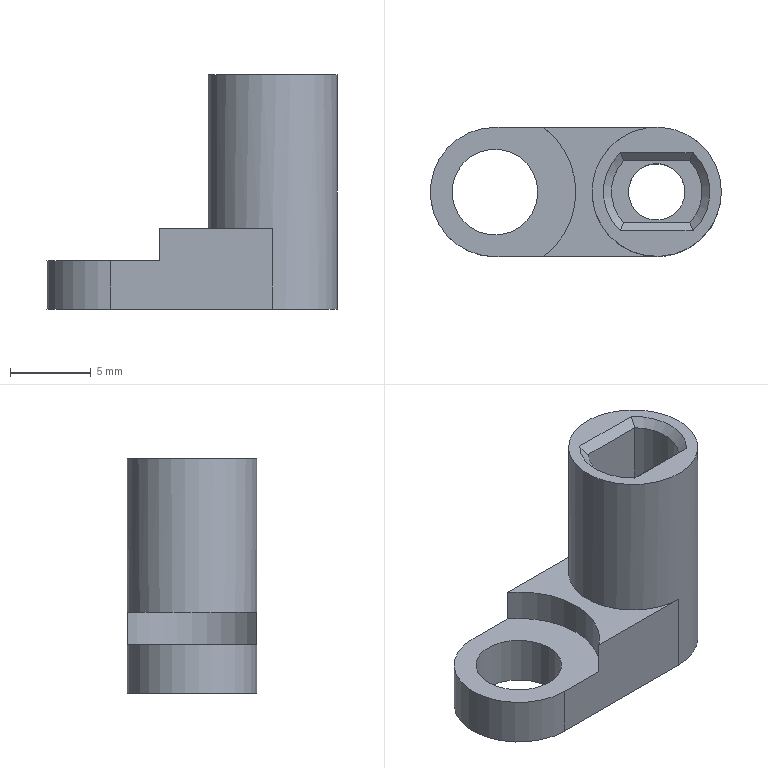Part | NX | features BREP 1 | 1 solid | 22 faces | box 18 x 8 x 14.5 mm | volume 713.021 mm3 | plane 12 | cylinder 8 | cone 2 | commonest cylinder face diameters 5.6 x2 8 x2 3.5 x1 5.3 x1 6 x1 10 x1
STEP:
#1=CARTESIAN_POINT('',(-20.737,0.,0.));
#2=VERTEX_POINT('',#1);
#3=CARTESIAN_POINT('',(-17.737,0.,0.));
#4=DIRECTION('',(0.,0.,-1.));
#5=DIRECTION('',(-1.,0.,0.));
#6=AXIS2_PLACEMENT_3D('',#3,#4,#5);
#7=CIRCLE('',#6,3.);
#8=EDGE_CURVE('',#2,#2,#7,.T.);
#9=ORIENTED_EDGE('',*,*,#8,.T.);
#10=EDGE_LOOP('',(#9));
#11=FACE_BOUND('',#10,.T.);
#12=CARTESIAN_POINT('',(-20.737,0.,2.));
#13=VERTEX_POINT('',#12);
#14=CARTESIAN_POINT('',(-17.737,0.,2.));
#15=DIRECTION('',(0.,0.,-1.));
#16=DIRECTION('',(-1.,0.,0.));
#17=AXIS2_PLACEMENT_3D('',#14,#15,#16);
#18=CIRCLE('',#17,3.);
#19=EDGE_CURVE('',#13,#13,#18,.T.);
#20=ORIENTED_EDGE('',*,*,#19,.F.);
#21=EDGE_LOOP('',(#20));
#22=FACE_BOUND('',#21,.T.);
#23=CARTESIAN_POINT('',(-17.737,0.,2.));
#24=DIRECTION('',(0.,0.,-1.));
#25=DIRECTION('',(1.,0.,0.));
#26=AXIS2_PLACEMENT_3D('',#23,#24,#25);
#27=CYLINDRICAL_SURFACE('',#26,3.);
#28=ADVANCED_FACE('',(#11,#22),#27,.F.);
#29=CARTESIAN_POINT('',(-24.737,-4.,3.));
#30=VERTEX_POINT('',#29);
#31=CARTESIAN_POINT('',(-24.737,4.,3.));
#32=VERTEX_POINT('',#31);
#33=CARTESIAN_POINT('',(-27.737,0.,3.));
#34=DIRECTION('',(0.,0.,1.));
#35=DIRECTION('',(1.,0.,0.));
#36=AXIS2_PLACEMENT_3D('',#33,#34,#35);
#37=CIRCLE('',#36,5.);
#38=EDGE_CURVE('',#30,#32,#37,.T.);
#39=ORIENTED_EDGE('',*,*,#38,.F.);
#40=CARTESIAN_POINT('',(-24.737,-4.,5.));
#41=VERTEX_POINT('',#40);
#42=CARTESIAN_POINT('',(-24.737,-4.,3.));
#43=DIRECTION('',(0.,0.,-1.));
#44=VECTOR('',#43,1000.);
#45=LINE('',#42,#44);
#46=EDGE_CURVE('',#41,#30,#45,.T.);
#47=ORIENTED_EDGE('',*,*,#46,.F.);
#48=CARTESIAN_POINT('',(-24.737,4.,5.));
#49=VERTEX_POINT('',#48);
#50=CARTESIAN_POINT('',(-27.737,0.,5.));
#51=DIRECTION('',(0.,0.,1.));
#52=DIRECTION('',(1.,0.,0.));
#53=AXIS2_PLACEMENT_3D('',#50,#51,#52);
#54=CIRCLE('',#53,5.);
#55=EDGE_CURVE('',#41,#49,#54,.T.);
#56=ORIENTED_EDGE('',*,*,#55,.T.);
#57=CARTESIAN_POINT('',(-24.737,4.,3.));
#58=DIRECTION('',(0.,0.,1.));
#59=VECTOR('',#58,1000.);
#60=LINE('',#57,#59);
#61=EDGE_CURVE('',#32,#49,#60,.T.);
#62=ORIENTED_EDGE('',*,*,#61,.F.);
#63=EDGE_LOOP('',(#39,#47,#56,#62));
#64=FACE_BOUND('',#63,.T.);
#65=CARTESIAN_POINT('',(-27.737,0.,3.));
#66=DIRECTION('',(0.,0.,1.));
#67=DIRECTION('',(-1.,0.,0.));
#68=AXIS2_PLACEMENT_3D('',#65,#66,#67);
#69=CYLINDRICAL_SURFACE('',#68,5.);
#70=ADVANCED_FACE('',(#64),#69,.F.);
#71=CARTESIAN_POINT('',(-15.693,-1.913,14.));
#72=VERTEX_POINT('',#71);
#73=CARTESIAN_POINT('',(-15.693,1.913,14.));
#74=VERTEX_POINT('',#73);
#75=CARTESIAN_POINT('',(-17.737,0.,14.));
#76=DIRECTION('',(0.,0.,1.));
#77=DIRECTION('',(1.,0.,0.));
#78=AXIS2_PLACEMENT_3D('',#75,#76,#77);
#79=CIRCLE('',#78,2.8);
#80=EDGE_CURVE('',#72,#74,#79,.T.);
#81=ORIENTED_EDGE('',*,*,#80,.F.);
#82=CARTESIAN_POINT('',(-15.487,-2.413,14.5));
#83=VERTEX_POINT('',#82);
#84=CARTESIAN_POINT('',(-15.487,-2.413,14.5));
#85=CARTESIAN_POINT('',(-15.552,-2.246,14.333));
#86=CARTESIAN_POINT('',(-15.621,-2.079,14.166));
#87=CARTESIAN_POINT('',(-15.693,-1.913,14.));
#88=B_SPLINE_CURVE_WITH_KNOTS('',3,(#84,#85,#86,#87),.UNSPECIFIED.,.F.,.F.,(4,4),(0.,1.),.PIECEWISE_BEZIER_KNOTS.);
#89=EDGE_CURVE('',#83,#72,#88,.T.);
#90=ORIENTED_EDGE('',*,*,#89,.F.);
#91=CARTESIAN_POINT('',(-15.487,2.413,14.5));
#92=VERTEX_POINT('',#91);
#93=CARTESIAN_POINT('',(-17.737,0.,14.5));
#94=DIRECTION('',(0.,0.,-1.));
#95=DIRECTION('',(1.,0.,0.));
#96=AXIS2_PLACEMENT_3D('',#93,#94,#95);
#97=CIRCLE('',#96,3.3);
#98=EDGE_CURVE('',#92,#83,#97,.T.);
#99=ORIENTED_EDGE('',*,*,#98,.F.);
#100=CARTESIAN_POINT('',(-15.693,1.913,14.));
#101=CARTESIAN_POINT('',(-15.621,2.079,14.166));
#102=CARTESIAN_POINT('',(-15.552,2.246,14.333));
#103=CARTESIAN_POINT('',(-15.487,2.413,14.5));
#104=B_SPLINE_CURVE_WITH_KNOTS('',3,(#100,#101,#102,#103),.UNSPECIFIED.,.F.,.F.,(4,4),(0.,1.),.PIECEWISE_BEZIER_KNOTS.);
#105=EDGE_CURVE('',#74,#92,#104,.T.);
#106=ORIENTED_EDGE('',*,*,#105,.F.);
#107=EDGE_LOOP('',(#81,#90,#99,#106));
#108=FACE_BOUND('',#107,.T.);
#109=CARTESIAN_POINT('',(-17.737,0.,14.));
#110=DIRECTION('',(0.,0.,1.));
#111=DIRECTION('',(-1.,0.,0.));
#112=AXIS2_PLACEMENT_3D('',#109,#110,#111);
#113=CONICAL_SURFACE('',#112,2.8,0.7854);
#114=ADVANCED_FACE('',(#108),#113,.F.);
#115=CARTESIAN_POINT('',(-15.693,-1.913,9.5));
#116=VERTEX_POINT('',#115);
#117=CARTESIAN_POINT('',(-15.693,1.913,9.5));
#118=VERTEX_POINT('',#117);
#119=CARTESIAN_POINT('',(-17.737,0.,9.5));
#120=DIRECTION('',(0.,0.,1.));
#121=DIRECTION('',(1.,0.,0.));
#122=AXIS2_PLACEMENT_3D('',#119,#120,#121);
#123=CIRCLE('',#122,2.8);
#124=EDGE_CURVE('',#116,#118,#123,.T.);
#125=ORIENTED_EDGE('',*,*,#124,.F.);
#126=CARTESIAN_POINT('',(-15.693,-1.913,9.5));
#127=DIRECTION('',(0.,0.,1.));
#128=VECTOR('',#127,1000.);
#129=LINE('',#126,#128);
#130=EDGE_CURVE('',#116,#72,#129,.T.);
#131=ORIENTED_EDGE('',*,*,#130,.T.);
#132=ORIENTED_EDGE('',*,*,#80,.T.);
#133=CARTESIAN_POINT('',(-15.693,1.913,9.5));
#134=DIRECTION('',(0.,0.,1.));
#135=VECTOR('',#134,1000.);
#136=LINE('',#133,#135);
#137=EDGE_CURVE('',#118,#74,#136,.T.);
#138=ORIENTED_EDGE('',*,*,#137,.F.);
#139=EDGE_LOOP('',(#125,#131,#132,#138));
#140=FACE_BOUND('',#139,.T.);
#141=CARTESIAN_POINT('',(-17.737,0.,9.5));
#142=DIRECTION('',(0.,0.,1.));
#143=DIRECTION('',(-1.,0.,0.));
#144=AXIS2_PLACEMENT_3D('',#141,#142,#143);
#145=CYLINDRICAL_SURFACE('',#144,2.8);
#146=ADVANCED_FACE('',(#140),#145,.F.);
#147=CARTESIAN_POINT('',(-17.737,4.,5.));
#148=VERTEX_POINT('',#147);
#149=CARTESIAN_POINT('',(-17.737,-4.,5.));
#150=VERTEX_POINT('',#149);
#151=CARTESIAN_POINT('',(-17.737,0.,5.));
#152=DIRECTION('',(0.,0.,1.));
#153=DIRECTION('',(1.,0.,0.));
#154=AXIS2_PLACEMENT_3D('',#151,#152,#153);
#155=CIRCLE('',#154,4.);
#156=EDGE_CURVE('',#148,#150,#155,.T.);
#157=ORIENTED_EDGE('',*,*,#156,.T.);
#158=CARTESIAN_POINT('',(-17.737,-4.,0.));
#159=VERTEX_POINT('',#158);
#160=CARTESIAN_POINT('',(-17.737,-4.,5.));
#161=DIRECTION('',(0.,0.,-1.));
#162=VECTOR('',#161,1000.);
#163=LINE('',#160,#162);
#164=EDGE_CURVE('',#150,#159,#163,.T.);
#165=ORIENTED_EDGE('',*,*,#164,.T.);
#166=CARTESIAN_POINT('',(-17.737,4.,0.));
#167=VERTEX_POINT('',#166);
#168=CARTESIAN_POINT('',(-17.737,0.,0.));
#169=DIRECTION('',(0.,0.,1.));
#170=DIRECTION('',(1.,0.,0.));
#171=AXIS2_PLACEMENT_3D('',#168,#169,#170);
#172=CIRCLE('',#171,4.);
#173=EDGE_CURVE('',#159,#167,#172,.T.);
#174=ORIENTED_EDGE('',*,*,#173,.T.);
#175=CARTESIAN_POINT('',(-17.737,4.,5.));
#176=DIRECTION('',(0.,0.,-1.));
#177=VECTOR('',#176,1000.);
#178=LINE('',#175,#177);
#179=EDGE_CURVE('',#148,#167,#178,.T.);
#180=ORIENTED_EDGE('',*,*,#179,.F.);
#181=EDGE_LOOP('',(#157,#165,#174,#180));
#182=FACE_BOUND('',#181,.T.);
#183=CARTESIAN_POINT('',(-13.737,0.,14.5));
#184=VERTEX_POINT('',#183);
#185=CARTESIAN_POINT('',(-17.737,0.,14.5));
#186=DIRECTION('',(0.,0.,1.));
#187=DIRECTION('',(1.,0.,0.));
#188=AXIS2_PLACEMENT_3D('',#185,#186,#187);
#189=CIRCLE('',#188,4.);
#190=EDGE_CURVE('',#184,#184,#189,.T.);
#191=ORIENTED_EDGE('',*,*,#190,.F.);
#192=EDGE_LOOP('',(#191));
#193=FACE_BOUND('',#192,.T.);
#194=CARTESIAN_POINT('',(-17.737,0.,5.));
#195=DIRECTION('',(0.,0.,-1.));
#196=DIRECTION('',(1.,0.,0.));
#197=AXIS2_PLACEMENT_3D('',#194,#195,#196);
#198=CYLINDRICAL_SURFACE('',#197,4.);
#199=ADVANCED_FACE('',(#182,#193),#198,.T.);
#200=CARTESIAN_POINT('',(-25.087,0.,3.));
#201=VERTEX_POINT('',#200);
#202=CARTESIAN_POINT('',(-27.737,0.,3.));
#203=DIRECTION('',(0.,0.,-1.));
#204=DIRECTION('',(1.,0.,0.));
#205=AXIS2_PLACEMENT_3D('',#202,#203,#204);
#206=CIRCLE('',#205,2.65);
#207=EDGE_CURVE('',#201,#201,#206,.T.);
#208=ORIENTED_EDGE('',*,*,#207,.F.);
#209=EDGE_LOOP('',(#208));
#210=FACE_BOUND('',#209,.T.);
#211=CARTESIAN_POINT('',(-25.087,0.,0.));
#212=VERTEX_POINT('',#211);
#213=CARTESIAN_POINT('',(-27.737,0.,0.));
#214=DIRECTION('',(0.,0.,1.));
#215=DIRECTION('',(1.,0.,0.));
#216=AXIS2_PLACEMENT_3D('',#213,#214,#215);
#217=CIRCLE('',#216,2.65);
#218=EDGE_CURVE('',#212,#212,#217,.T.);
#219=ORIENTED_EDGE('',*,*,#218,.F.);
#220=EDGE_LOOP('',(#219));
#221=FACE_BOUND('',#220,.T.);
#222=CARTESIAN_POINT('',(-27.737,0.,-3.));
#223=DIRECTION('',(0.,0.,1.));
#224=DIRECTION('',(-1.,0.,0.));
#225=AXIS2_PLACEMENT_3D('',#222,#223,#224);
#226=CYLINDRICAL_SURFACE('',#225,2.65);
#227=ADVANCED_FACE('',(#210,#221),#226,.F.);
#228=CARTESIAN_POINT('',(-27.737,4.,3.));
#229=VERTEX_POINT('',#228);
#230=CARTESIAN_POINT('',(-27.737,-4.,3.));
#231=VERTEX_POINT('',#230);
#232=CARTESIAN_POINT('',(-27.737,0.,3.));
#233=DIRECTION('',(0.,0.,1.));
#234=DIRECTION('',(1.,0.,0.));
#235=AXIS2_PLACEMENT_3D('',#232,#233,#234);
#236=CIRCLE('',#235,4.);
#237=EDGE_CURVE('',#229,#231,#236,.T.);
#238=ORIENTED_EDGE('',*,*,#237,.F.);
#239=CARTESIAN_POINT('',(-27.737,4.,0.));
#240=VERTEX_POINT('',#239);
#241=CARTESIAN_POINT('',(-27.737,4.,5.));
#242=DIRECTION('',(0.,0.,-1.));
#243=VECTOR('',#242,1000.);
#244=LINE('',#241,#243);
#245=EDGE_CURVE('',#229,#240,#244,.T.);
#246=ORIENTED_EDGE('',*,*,#245,.T.);
#247=CARTESIAN_POINT('',(-27.737,-4.,0.));
#248=VERTEX_POINT('',#247);
#249=CARTESIAN_POINT('',(-27.737,0.,0.));
#250=DIRECTION('',(0.,0.,1.));
#251=DIRECTION('',(1.,0.,0.));
#252=AXIS2_PLACEMENT_3D('',#249,#250,#251);
#253=CIRCLE('',#252,4.);
#254=EDGE_CURVE('',#240,#248,#253,.T.);
#255=ORIENTED_EDGE('',*,*,#254,.T.);
#256=CARTESIAN_POINT('',(-27.737,-4.,5.));
#257=DIRECTION('',(0.,0.,-1.));
#258=VECTOR('',#257,1000.);
#259=LINE('',#256,#258);
#260=EDGE_CURVE('',#231,#248,#259,.T.);
#261=ORIENTED_EDGE('',*,*,#260,.F.);
#262=EDGE_LOOP('',(#238,#246,#255,#261));
#263=FACE_BOUND('',#262,.T.);
#264=CARTESIAN_POINT('',(-27.737,0.,5.));
#265=DIRECTION('',(0.,0.,-1.));
#266=DIRECTION('',(1.,0.,0.));
#267=AXIS2_PLACEMENT_3D('',#264,#265,#266);
#268=CYLINDRICAL_SURFACE('',#267,4.);
#269=ADVANCED_FACE('',(#263),#268,.T.);
#270=CARTESIAN_POINT('',(-15.987,0.,9.5));
#271=VERTEX_POINT('',#270);
#272=CARTESIAN_POINT('',(-17.737,0.,9.5));
#273=DIRECTION('',(0.,0.,1.));
#274=DIRECTION('',(1.,0.,0.));
#275=AXIS2_PLACEMENT_3D('',#272,#273,#274);
#276=CIRCLE('',#275,1.75);
#277=EDGE_CURVE('',#271,#271,#276,.T.);
#278=ORIENTED_EDGE('',*,*,#277,.T.);
#279=EDGE_LOOP('',(#278));
#280=FACE_BOUND('',#279,.T.);
#281=CARTESIAN_POINT('',(-19.487,0.,2.));
#282=VERTEX_POINT('',#281);
#283=CARTESIAN_POINT('',(-17.737,0.,2.));
#284=DIRECTION('',(0.,0.,1.));
#285=DIRECTION('',(-1.,0.,0.));
#286=AXIS2_PLACEMENT_3D('',#283,#284,#285);
#287=CIRCLE('',#286,1.75);
#288=EDGE_CURVE('',#282,#282,#287,.T.);
#289=ORIENTED_EDGE('',*,*,#288,.F.);
#290=EDGE_LOOP('',(#289));
#291=FACE_BOUND('',#290,.T.);
#292=CARTESIAN_POINT('',(-17.737,0.,-4.95));
#293=DIRECTION('',(0.,0.,1.));
#294=DIRECTION('',(-1.,0.,0.));
#295=AXIS2_PLACEMENT_3D('',#292,#293,#294);
#296=CYLINDRICAL_SURFACE('',#295,1.75);
#297=ADVANCED_FACE('',(#280,#291),#296,.F.);
#298=CARTESIAN_POINT('',(-27.737,-4.,5.));
#299=DIRECTION('',(1.,0.,0.));
#300=VECTOR('',#299,1000.);
#301=LINE('',#298,#300);
#302=EDGE_CURVE('',#41,#150,#301,.T.);
#303=ORIENTED_EDGE('',*,*,#302,.F.);
#304=ORIENTED_EDGE('',*,*,#46,.T.);
#305=CARTESIAN_POINT('',(-27.737,-4.,3.));
#306=DIRECTION('',(1.,0.,0.));
#307=VECTOR('',#306,1000.);
#308=LINE('',#305,#307);
#309=EDGE_CURVE('',#231,#30,#308,.T.);
#310=ORIENTED_EDGE('',*,*,#309,.F.);
#311=ORIENTED_EDGE('',*,*,#260,.T.);
#312=CARTESIAN_POINT('',(-27.737,-4.,0.));
#313=DIRECTION('',(1.,0.,0.));
#314=VECTOR('',#313,1000.);
#315=LINE('',#312,#314);
#316=EDGE_CURVE('',#248,#159,#315,.T.);
#317=ORIENTED_EDGE('',*,*,#316,.T.);
#318=ORIENTED_EDGE('',*,*,#164,.F.);
#319=EDGE_LOOP('',(#303,#304,#310,#311,#317,#318));
#320=FACE_BOUND('',#319,.T.);
#321=CARTESIAN_POINT('',(-27.737,-4.,5.));
#322=DIRECTION('',(0.,1.,0.));
#323=DIRECTION('',(0.,0.,-1.));
#324=AXIS2_PLACEMENT_3D('',#321,#322,#323);
#325=PLANE('',#324);
#326=ADVANCED_FACE('',(#320),#325,.F.);
#327=CARTESIAN_POINT('',(-27.737,4.,3.));
#328=DIRECTION('',(-1.,0.,0.));
#329=VECTOR('',#328,1000.);
#330=LINE('',#327,#329);
#331=EDGE_CURVE('',#32,#229,#330,.T.);
#332=ORIENTED_EDGE('',*,*,#331,.F.);
#333=ORIENTED_EDGE('',*,*,#61,.T.);
#334=CARTESIAN_POINT('',(-27.737,4.,5.));
#335=DIRECTION('',(-1.,0.,0.));
#336=VECTOR('',#335,1000.);
#337=LINE('',#334,#336);
#338=EDGE_CURVE('',#148,#49,#337,.T.);
#339=ORIENTED_EDGE('',*,*,#338,.F.);
#340=ORIENTED_EDGE('',*,*,#179,.T.);
#341=CARTESIAN_POINT('',(-27.737,4.,0.));
#342=DIRECTION('',(-1.,0.,0.));
#343=VECTOR('',#342,1000.);
#344=LINE('',#341,#343);
#345=EDGE_CURVE('',#167,#240,#344,.T.);
#346=ORIENTED_EDGE('',*,*,#345,.T.);
#347=ORIENTED_EDGE('',*,*,#245,.F.);
#348=EDGE_LOOP('',(#332,#333,#339,#340,#346,#347));
#349=FACE_BOUND('',#348,.T.);
#350=CARTESIAN_POINT('',(-27.737,4.,5.));
#351=DIRECTION('',(0.,-1.,0.));
#352=DIRECTION('',(0.,0.,1.));
#353=AXIS2_PLACEMENT_3D('',#350,#351,#352);
#354=PLANE('',#353);
#355=ADVANCED_FACE('',(#349),#354,.F.);
#356=ORIENTED_EDGE('',*,*,#55,.F.);
#357=ORIENTED_EDGE('',*,*,#302,.T.);
#358=ORIENTED_EDGE('',*,*,#156,.F.);
#359=ORIENTED_EDGE('',*,*,#338,.T.);
#360=EDGE_LOOP('',(#356,#357,#358,#359));
#361=FACE_BOUND('',#360,.T.);
#362=CARTESIAN_POINT('',(-27.737,0.,5.));
#363=DIRECTION('',(0.,0.,1.));
#364=DIRECTION('',(-1.,0.,0.));
#365=AXIS2_PLACEMENT_3D('',#362,#363,#364);
#366=PLANE('',#365);
#367=ADVANCED_FACE('',(#361),#366,.T.);
#368=ORIENTED_EDGE('',*,*,#8,.F.);
#369=EDGE_LOOP('',(#368));
#370=FACE_BOUND('',#369,.T.);
#371=ORIENTED_EDGE('',*,*,#218,.T.);
#372=EDGE_LOOP('',(#371));
#373=FACE_BOUND('',#372,.T.);
#374=ORIENTED_EDGE('',*,*,#254,.F.);
#375=ORIENTED_EDGE('',*,*,#345,.F.);
#376=ORIENTED_EDGE('',*,*,#173,.F.);
#377=ORIENTED_EDGE('',*,*,#316,.F.);
#378=EDGE_LOOP('',(#374,#375,#376,#377));
#379=FACE_BOUND('',#378,.T.);
#380=CARTESIAN_POINT('',(-27.737,0.,0.));
#381=DIRECTION('',(0.,0.,1.));
#382=DIRECTION('',(-1.,0.,0.));
#383=AXIS2_PLACEMENT_3D('',#380,#381,#382);
#384=PLANE('',#383);
#385=ADVANCED_FACE('',(#370,#373,#379),#384,.F.);
#386=CARTESIAN_POINT('',(-19.988,-2.413,14.5));
#387=VERTEX_POINT('',#386);
#388=CARTESIAN_POINT('',(-19.782,-2.413,14.5));
#389=DIRECTION('',(-1.,0.,0.));
#390=VECTOR('',#389,1000.);
#391=LINE('',#388,#390);
#392=EDGE_CURVE('',#83,#387,#391,.T.);
#393=ORIENTED_EDGE('',*,*,#392,.T.);
#394=CARTESIAN_POINT('',(-19.988,2.413,14.5));
#395=VERTEX_POINT('',#394);
#396=CARTESIAN_POINT('',(-17.737,0.,14.5));
#397=DIRECTION('',(0.,0.,-1.));
#398=DIRECTION('',(1.,0.,0.));
#399=AXIS2_PLACEMENT_3D('',#396,#397,#398);
#400=CIRCLE('',#399,3.3);
#401=EDGE_CURVE('',#387,#395,#400,.T.);
#402=ORIENTED_EDGE('',*,*,#401,.T.);
#403=CARTESIAN_POINT('',(-15.693,2.413,14.5));
#404=DIRECTION('',(1.,0.,0.));
#405=VECTOR('',#404,1000.);
#406=LINE('',#403,#405);
#407=EDGE_CURVE('',#395,#92,#406,.T.);
#408=ORIENTED_EDGE('',*,*,#407,.T.);
#409=ORIENTED_EDGE('',*,*,#98,.T.);
#410=EDGE_LOOP('',(#393,#402,#408,#409));
#411=FACE_BOUND('',#410,.T.);
#412=ORIENTED_EDGE('',*,*,#190,.T.);
#413=EDGE_LOOP('',(#412));
#414=FACE_BOUND('',#413,.T.);
#415=CARTESIAN_POINT('',(-17.737,0.,14.5));
#416=DIRECTION('',(0.,0.,1.));
#417=DIRECTION('',(-1.,0.,0.));
#418=AXIS2_PLACEMENT_3D('',#415,#416,#417);
#419=PLANE('',#418);
#420=ADVANCED_FACE('',(#411,#414),#419,.T.);
#421=CARTESIAN_POINT('',(-19.782,1.913,9.5));
#422=VERTEX_POINT('',#421);
#423=CARTESIAN_POINT('',(-19.782,1.913,14.));
#424=VERTEX_POINT('',#423);
#425=CARTESIAN_POINT('',(-19.782,1.913,9.5));
#426=DIRECTION('',(0.,0.,1.));
#427=VECTOR('',#426,1000.);
#428=LINE('',#425,#427);
#429=EDGE_CURVE('',#422,#424,#428,.T.);
#430=ORIENTED_EDGE('',*,*,#429,.T.);
#431=CARTESIAN_POINT('',(-19.782,-1.913,14.));
#432=VERTEX_POINT('',#431);
#433=CARTESIAN_POINT('',(-17.737,0.,14.));
#434=DIRECTION('',(0.,0.,1.));
#435=DIRECTION('',(1.,0.,0.));
#436=AXIS2_PLACEMENT_3D('',#433,#434,#435);
#437=CIRCLE('',#436,2.8);
#438=EDGE_CURVE('',#424,#432,#437,.T.);
#439=ORIENTED_EDGE('',*,*,#438,.T.);
#440=CARTESIAN_POINT('',(-19.782,-1.913,9.5));
#441=VERTEX_POINT('',#440);
#442=CARTESIAN_POINT('',(-19.782,-1.913,9.5));
#443=DIRECTION('',(0.,0.,1.));
#444=VECTOR('',#443,1000.);
#445=LINE('',#442,#444);
#446=EDGE_CURVE('',#441,#432,#445,.T.);
#447=ORIENTED_EDGE('',*,*,#446,.F.);
#448=CARTESIAN_POINT('',(-17.737,0.,9.5));
#449=DIRECTION('',(0.,0.,1.));
#450=DIRECTION('',(1.,0.,0.));
#451=AXIS2_PLACEMENT_3D('',#448,#449,#450);
#452=CIRCLE('',#451,2.8);
#453=EDGE_CURVE('',#422,#441,#452,.T.);
#454=ORIENTED_EDGE('',*,*,#453,.F.);
#455=EDGE_LOOP('',(#430,#439,#447,#454));
#456=FACE_BOUND('',#455,.T.);
#457=CARTESIAN_POINT('',(-17.737,0.,9.5));
#458=DIRECTION('',(0.,0.,1.));
#459=DIRECTION('',(-1.,0.,0.));
#460=AXIS2_PLACEMENT_3D('',#457,#458,#459);
#461=CYLINDRICAL_SURFACE('',#460,2.8);
#462=ADVANCED_FACE('',(#456),#461,.F.);
#463=ORIENTED_EDGE('',*,*,#137,.T.);
#464=CARTESIAN_POINT('',(-19.782,1.913,14.));
#465=DIRECTION('',(-1.,0.,0.));
#466=VECTOR('',#465,1000.);
#467=LINE('',#464,#466);
#468=EDGE_CURVE('',#74,#424,#467,.T.);
#469=ORIENTED_EDGE('',*,*,#468,.T.);
#470=ORIENTED_EDGE('',*,*,#429,.F.);
#471=CARTESIAN_POINT('',(-19.782,1.913,9.5));
#472=DIRECTION('',(-1.,0.,0.));
#473=VECTOR('',#472,1000.);
#474=LINE('',#471,#473);
#475=EDGE_CURVE('',#118,#422,#474,.T.);
#476=ORIENTED_EDGE('',*,*,#475,.F.);
#477=EDGE_LOOP('',(#463,#469,#470,#476));
#478=FACE_BOUND('',#477,.T.);
#479=CARTESIAN_POINT('',(-19.782,1.913,9.5));
#480=DIRECTION('',(0.,1.,0.));
#481=DIRECTION('',(0.,0.,-1.));
#482=AXIS2_PLACEMENT_3D('',#479,#480,#481);
#483=PLANE('',#482);
#484=ADVANCED_FACE('',(#478),#483,.F.);
#485=ORIENTED_EDGE('',*,*,#446,.T.);
#486=CARTESIAN_POINT('',(-15.693,-1.913,14.));
#487=DIRECTION('',(1.,0.,0.));
#488=VECTOR('',#487,1000.);
#489=LINE('',#486,#488);
#490=EDGE_CURVE('',#432,#72,#489,.T.);
#491=ORIENTED_EDGE('',*,*,#490,.T.);
#492=ORIENTED_EDGE('',*,*,#130,.F.);
#493=CARTESIAN_POINT('',(-19.782,-1.913,9.5));
#494=DIRECTION('',(1.,0.,0.));
#495=VECTOR('',#494,1000.);
#496=LINE('',#493,#495);
#497=EDGE_CURVE('',#441,#116,#496,.T.);
#498=ORIENTED_EDGE('',*,*,#497,.F.);
#499=EDGE_LOOP('',(#485,#491,#492,#498));
#500=FACE_BOUND('',#499,.T.);
#501=CARTESIAN_POINT('',(-19.782,-1.913,9.5));
#502=DIRECTION('',(0.,-1.,0.));
#503=DIRECTION('',(0.,0.,1.));
#504=AXIS2_PLACEMENT_3D('',#501,#502,#503);
#505=PLANE('',#504);
#506=ADVANCED_FACE('',(#500),#505,.F.);
#507=ORIENTED_EDGE('',*,*,#277,.F.);
#508=EDGE_LOOP('',(#507));
#509=FACE_BOUND('',#508,.T.);
#510=ORIENTED_EDGE('',*,*,#453,.T.);
#511=ORIENTED_EDGE('',*,*,#497,.T.);
#512=ORIENTED_EDGE('',*,*,#124,.T.);
#513=ORIENTED_EDGE('',*,*,#475,.T.);
#514=EDGE_LOOP('',(#510,#511,#512,#513));
#515=FACE_BOUND('',#514,.T.);
#516=CARTESIAN_POINT('',(-17.737,0.,9.5));
#517=DIRECTION('',(0.,0.,1.));
#518=DIRECTION('',(-1.,0.,0.));
#519=AXIS2_PLACEMENT_3D('',#516,#517,#518);
#520=PLANE('',#519);
#521=ADVANCED_FACE('',(#509,#515),#520,.T.);
#522=ORIENTED_EDGE('',*,*,#105,.T.);
#523=ORIENTED_EDGE('',*,*,#407,.F.);
#524=CARTESIAN_POINT('',(-19.782,1.913,14.));
#525=CARTESIAN_POINT('',(-19.854,2.079,14.166));
#526=CARTESIAN_POINT('',(-19.922,2.246,14.333));
#527=CARTESIAN_POINT('',(-19.988,2.413,14.5));
#528=B_SPLINE_CURVE_WITH_KNOTS('',3,(#524,#525,#526,#527),.UNSPECIFIED.,.F.,.F.,(4,4),(0.,1.),.PIECEWISE_BEZIER_KNOTS.);
#529=EDGE_CURVE('',#424,#395,#528,.T.);
#530=ORIENTED_EDGE('',*,*,#529,.F.);
#531=ORIENTED_EDGE('',*,*,#468,.F.);
#532=EDGE_LOOP('',(#522,#523,#530,#531));
#533=FACE_BOUND('',#532,.T.);
#534=CARTESIAN_POINT('',(-19.782,1.913,14.));
#535=DIRECTION('',(0.,-0.7071,0.7071));
#536=DIRECTION('',(-1.,0.,0.));
#537=AXIS2_PLACEMENT_3D('',#534,#535,#536);
#538=PLANE('',#537);
#539=ADVANCED_FACE('',(#533),#538,.T.);
#540=ORIENTED_EDGE('',*,*,#89,.T.);
#541=ORIENTED_EDGE('',*,*,#490,.F.);
#542=CARTESIAN_POINT('',(-19.988,-2.413,14.5));
#543=CARTESIAN_POINT('',(-19.922,-2.246,14.333));
#544=CARTESIAN_POINT('',(-19.854,-2.079,14.166));
#545=CARTESIAN_POINT('',(-19.782,-1.913,14.));
#546=B_SPLINE_CURVE_WITH_KNOTS('',3,(#542,#543,#544,#545),.UNSPECIFIED.,.F.,.F.,(4,4),(0.,1.),.PIECEWISE_BEZIER_KNOTS.);
#547=EDGE_CURVE('',#387,#432,#546,.T.);
#548=ORIENTED_EDGE('',*,*,#547,.F.);
#549=ORIENTED_EDGE('',*,*,#392,.F.);
#550=EDGE_LOOP('',(#540,#541,#548,#549));
#551=FACE_BOUND('',#550,.T.);
#552=CARTESIAN_POINT('',(-19.782,-1.913,14.));
#553=DIRECTION('',(0.,0.7071,0.7071));
#554=DIRECTION('',(1.,0.,0.));
#555=AXIS2_PLACEMENT_3D('',#552,#553,#554);
#556=PLANE('',#555);
#557=ADVANCED_FACE('',(#551),#556,.T.);
#558=ORIENTED_EDGE('',*,*,#529,.T.);
#559=ORIENTED_EDGE('',*,*,#401,.F.);
#560=ORIENTED_EDGE('',*,*,#547,.T.);
#561=ORIENTED_EDGE('',*,*,#438,.F.);
#562=EDGE_LOOP('',(#558,#559,#560,#561));
#563=FACE_BOUND('',#562,.T.);
#564=CARTESIAN_POINT('',(-17.737,0.,14.));
#565=DIRECTION('',(0.,0.,1.));
#566=DIRECTION('',(-1.,0.,0.));
#567=AXIS2_PLACEMENT_3D('',#564,#565,#566);
#568=CONICAL_SURFACE('',#567,2.8,0.7854);
#569=ADVANCED_FACE('',(#563),#568,.F.);
#570=ORIENTED_EDGE('',*,*,#207,.T.);
#571=EDGE_LOOP('',(#570));
#572=FACE_BOUND('',#571,.T.);
#573=ORIENTED_EDGE('',*,*,#309,.T.);
#574=ORIENTED_EDGE('',*,*,#38,.T.);
#575=ORIENTED_EDGE('',*,*,#331,.T.);
#576=ORIENTED_EDGE('',*,*,#237,.T.);
#577=EDGE_LOOP('',(#573,#574,#575,#576));
#578=FACE_BOUND('',#577,.T.);
#579=CARTESIAN_POINT('',(-27.737,0.,3.));
#580=DIRECTION('',(0.,0.,1.));
#581=DIRECTION('',(-1.,0.,0.));
#582=AXIS2_PLACEMENT_3D('',#579,#580,#581);
#583=PLANE('',#582);
#584=ADVANCED_FACE('',(#572,#578),#583,.T.);
#585=ORIENTED_EDGE('',*,*,#19,.T.);
#586=EDGE_LOOP('',(#585));
#587=FACE_BOUND('',#586,.T.);
#588=ORIENTED_EDGE('',*,*,#288,.T.);
#589=EDGE_LOOP('',(#588));
#590=FACE_BOUND('',#589,.T.);
#591=CARTESIAN_POINT('',(-17.737,0.,2.));
#592=DIRECTION('',(0.,0.,-1.));
#593=DIRECTION('',(1.,0.,0.));
#594=AXIS2_PLACEMENT_3D('',#591,#592,#593);
#595=PLANE('',#594);
#596=ADVANCED_FACE('',(#587,#590),#595,.T.);
#597=CLOSED_SHELL('',(#28,#70,#114,#146,#199,#227,#269,#297,#326,#355,#367,#385,#420,#462,#484,#506,#521,#539,#557,#569,#584,#596));
#598=MANIFOLD_SOLID_BREP('',#597);
#599=(LENGTH_UNIT()NAMED_UNIT(*)SI_UNIT(.MILLI.,.METRE.));
#600=UNCERTAINTY_MEASURE_WITH_UNIT(LENGTH_MEASURE(0.00001),#599,'','');
#601=(NAMED_UNIT(*)PLANE_ANGLE_UNIT()SI_UNIT($,.RADIAN.));
#602=(NAMED_UNIT(*)SI_UNIT($,.STERADIAN.)SOLID_ANGLE_UNIT());
#603=(GEOMETRIC_REPRESENTATION_CONTEXT(3)GLOBAL_UNCERTAINTY_ASSIGNED_CONTEXT((#600))GLOBAL_UNIT_ASSIGNED_CONTEXT((#599,#601,#602))REPRESENTATION_CONTEXT('',''));
#604=ADVANCED_BREP_SHAPE_REPRESENTATION('',(#598),#603);